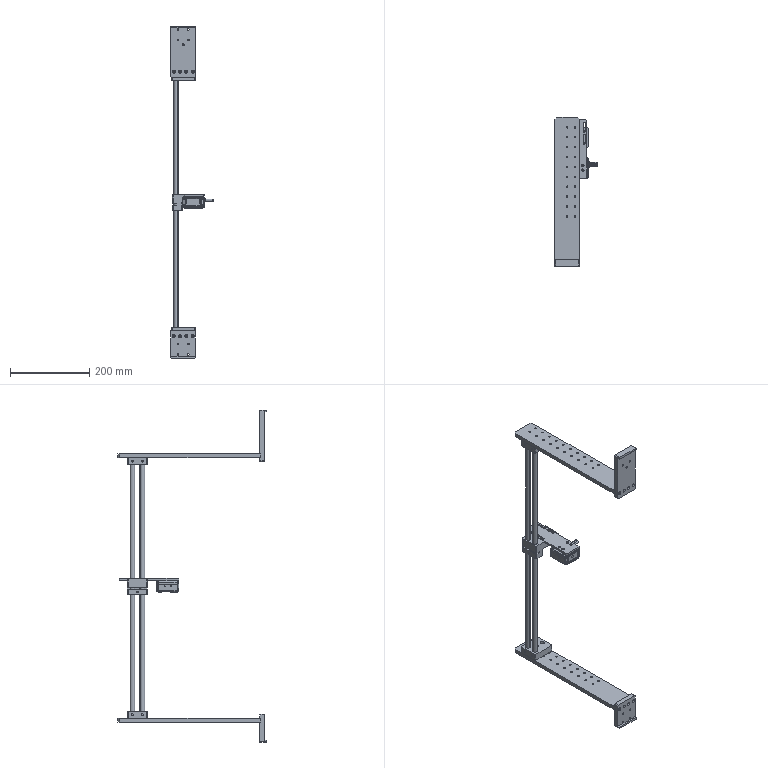Part | SolidWorks | 33 solids | 3178 faces | volume 984792 mm3 | cylinder 1212 | plane 1013 | spline 492 | cone 234 | torus 169 | sphere 58 | commonest cylinder face diameters 1.713 x174 1.376 x124 4 x107 4.2 x100 8 x70 1 x68